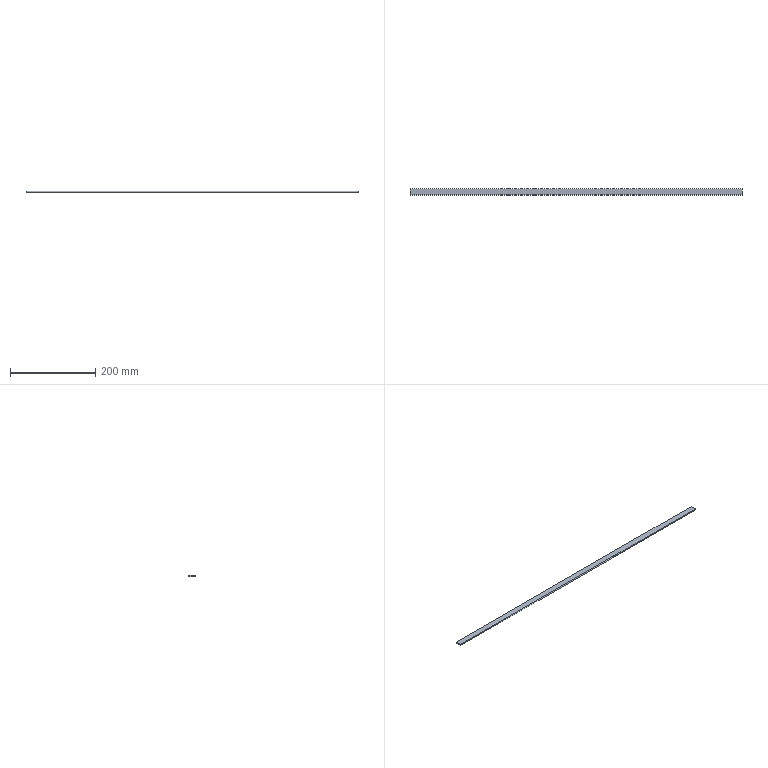Part | SolidWorks | features FlatPattern 1, Hem 1, SMBaseFlange 1, SheetMetal 1 | 1 solid | 14 faces | box 777 x 15 x 2.7 mm | volume 27651 mm3 | plane 12 | cylinder 2 | commonest cylinder face diameters 0.3 x1 2.7 x1
STEP:
#1=CARTESIAN_POINT('',(534.221,12.222,0.));
#2=VERTEX_POINT('',#1);
#3=CARTESIAN_POINT('',(534.221,25.872,0.));
#4=VERTEX_POINT('',#3);
#5=CARTESIAN_POINT('',(534.221,25.872,0.));
#6=DIRECTION('',(0.,1.,0.));
#7=VECTOR('',#6,1000.);
#8=LINE('',#5,#7);
#9=EDGE_CURVE('',#2,#4,#8,.T.);
#10=ORIENTED_EDGE('',*,*,#9,.F.);
#11=CARTESIAN_POINT('',(534.221,12.222,-1.2));
#12=VERTEX_POINT('',#11);
#13=CARTESIAN_POINT('',(534.221,12.222,0.));
#14=DIRECTION('',(0.,0.,-1.));
#15=VECTOR('',#14,1000.);
#16=LINE('',#13,#15);
#17=EDGE_CURVE('',#2,#12,#16,.T.);
#18=ORIENTED_EDGE('',*,*,#17,.T.);
#19=CARTESIAN_POINT('',(534.221,25.872,-1.2));
#20=VERTEX_POINT('',#19);
#21=CARTESIAN_POINT('',(534.221,25.872,-1.2));
#22=DIRECTION('',(0.,1.,0.));
#23=VECTOR('',#22,1000.);
#24=LINE('',#21,#23);
#25=EDGE_CURVE('',#12,#20,#24,.T.);
#26=ORIENTED_EDGE('',*,*,#25,.T.);
#27=CARTESIAN_POINT('',(534.221,25.872,-1.2));
#28=DIRECTION('',(0.,0.,1.));
#29=VECTOR('',#28,1000.);
#30=LINE('',#27,#29);
#31=EDGE_CURVE('',#20,#4,#30,.T.);
#32=ORIENTED_EDGE('',*,*,#31,.T.);
#33=EDGE_LOOP('',(#10,#18,#26,#32));
#34=FACE_OUTER_BOUND('',#33,.T.);
#35=CARTESIAN_POINT('',(534.221,25.872,-1.2));
#36=DIRECTION('',(1.,0.,0.));
#37=DIRECTION('',(0.,0.,-1.));
#38=AXIS2_PLACEMENT_3D('',#35,#36,#37);
#39=PLANE('',#38);
#40=ADVANCED_FACE('',(#34),#39,.T.);
#41=CARTESIAN_POINT('',(-242.779,12.222,0.));
#42=VERTEX_POINT('',#41);
#43=CARTESIAN_POINT('',(-242.779,12.222,-1.2));
#44=VERTEX_POINT('',#43);
#45=CARTESIAN_POINT('',(-242.779,12.222,0.));
#46=DIRECTION('',(0.,0.,-1.));
#47=VECTOR('',#46,1000.);
#48=LINE('',#45,#47);
#49=EDGE_CURVE('',#42,#44,#48,.T.);
#50=ORIENTED_EDGE('',*,*,#49,.F.);
#51=CARTESIAN_POINT('',(-242.779,25.872,0.));
#52=VERTEX_POINT('',#51);
#53=CARTESIAN_POINT('',(-242.779,25.872,0.));
#54=DIRECTION('',(0.,-1.,0.));
#55=VECTOR('',#54,1000.);
#56=LINE('',#53,#55);
#57=EDGE_CURVE('',#52,#42,#56,.T.);
#58=ORIENTED_EDGE('',*,*,#57,.F.);
#59=CARTESIAN_POINT('',(-242.779,25.872,-1.2));
#60=VERTEX_POINT('',#59);
#61=CARTESIAN_POINT('',(-242.779,25.872,-1.2));
#62=DIRECTION('',(0.,0.,1.));
#63=VECTOR('',#62,1000.);
#64=LINE('',#61,#63);
#65=EDGE_CURVE('',#60,#52,#64,.T.);
#66=ORIENTED_EDGE('',*,*,#65,.F.);
#67=CARTESIAN_POINT('',(-242.779,25.872,-1.2));
#68=DIRECTION('',(0.,-1.,0.));
#69=VECTOR('',#68,1000.);
#70=LINE('',#67,#69);
#71=EDGE_CURVE('',#60,#44,#70,.T.);
#72=ORIENTED_EDGE('',*,*,#71,.T.);
#73=EDGE_LOOP('',(#50,#58,#66,#72));
#74=FACE_OUTER_BOUND('',#73,.T.);
#75=CARTESIAN_POINT('',(-242.779,25.872,-1.2));
#76=DIRECTION('',(-1.,0.,0.));
#77=DIRECTION('',(0.,0.,1.));
#78=AXIS2_PLACEMENT_3D('',#75,#76,#77);
#79=PLANE('',#78);
#80=ADVANCED_FACE('',(#74),#79,.T.);
#81=CARTESIAN_POINT('',(-242.779,25.872,0.));
#82=DIRECTION('',(-1.,0.,0.));
#83=VECTOR('',#82,1000.);
#84=LINE('',#81,#83);
#85=EDGE_CURVE('',#4,#52,#84,.T.);
#86=ORIENTED_EDGE('',*,*,#85,.F.);
#87=ORIENTED_EDGE('',*,*,#31,.F.);
#88=CARTESIAN_POINT('',(-242.779,25.872,-1.2));
#89=DIRECTION('',(-1.,0.,0.));
#90=VECTOR('',#89,1000.);
#91=LINE('',#88,#90);
#92=EDGE_CURVE('',#20,#60,#91,.T.);
#93=ORIENTED_EDGE('',*,*,#92,.T.);
#94=ORIENTED_EDGE('',*,*,#65,.T.);
#95=EDGE_LOOP('',(#86,#87,#93,#94));
#96=FACE_OUTER_BOUND('',#95,.T.);
#97=CARTESIAN_POINT('',(-242.779,25.872,-1.2));
#98=DIRECTION('',(0.,1.,0.));
#99=DIRECTION('',(0.,0.,1.));
#100=AXIS2_PLACEMENT_3D('',#97,#98,#99);
#101=PLANE('',#100);
#102=ADVANCED_FACE('',(#96),#101,.T.);
#103=ORIENTED_EDGE('',*,*,#25,.F.);
#104=CARTESIAN_POINT('',(534.221,12.222,-1.2));
#105=DIRECTION('',(-1.,0.,0.));
#106=VECTOR('',#105,1000.);
#107=LINE('',#104,#106);
#108=EDGE_CURVE('',#12,#44,#107,.T.);
#109=ORIENTED_EDGE('',*,*,#108,.T.);
#110=ORIENTED_EDGE('',*,*,#71,.F.);
#111=ORIENTED_EDGE('',*,*,#92,.F.);
#112=EDGE_LOOP('',(#103,#109,#110,#111));
#113=FACE_OUTER_BOUND('',#112,.T.);
#114=CARTESIAN_POINT('',(0.,0.,-1.2));
#115=DIRECTION('',(0.,0.,1.));
#116=DIRECTION('',(1.,0.,0.));
#117=AXIS2_PLACEMENT_3D('',#114,#115,#116);
#118=PLANE('',#117);
#119=ADVANCED_FACE('',(#113),#118,.F.);
#120=CARTESIAN_POINT('',(534.221,12.222,0.));
#121=DIRECTION('',(-1.,0.,0.));
#122=VECTOR('',#121,1000.);
#123=LINE('',#120,#122);
#124=EDGE_CURVE('',#2,#42,#123,.T.);
#125=ORIENTED_EDGE('',*,*,#124,.F.);
#126=ORIENTED_EDGE('',*,*,#9,.T.);
#127=ORIENTED_EDGE('',*,*,#85,.T.);
#128=ORIENTED_EDGE('',*,*,#57,.T.);
#129=EDGE_LOOP('',(#125,#126,#127,#128));
#130=FACE_OUTER_BOUND('',#129,.T.);
#131=CARTESIAN_POINT('',(0.,0.,0.));
#132=DIRECTION('',(0.,0.,1.));
#133=DIRECTION('',(1.,0.,0.));
#134=AXIS2_PLACEMENT_3D('',#131,#132,#133);
#135=PLANE('',#134);
#136=ADVANCED_FACE('',(#130),#135,.T.);
#137=CARTESIAN_POINT('',(534.221,12.222,0.3));
#138=VERTEX_POINT('',#137);
#139=CARTESIAN_POINT('',(534.221,12.222,1.5));
#140=VERTEX_POINT('',#139);
#141=CARTESIAN_POINT('',(534.221,12.222,1.5));
#142=DIRECTION('',(0.,0.,1.));
#143=VECTOR('',#142,1000.);
#144=LINE('',#141,#143);
#145=EDGE_CURVE('',#138,#140,#144,.T.);
#146=ORIENTED_EDGE('',*,*,#145,.F.);
#147=CARTESIAN_POINT('',(534.221,25.872,0.3));
#148=VERTEX_POINT('',#147);
#149=CARTESIAN_POINT('',(534.221,19.047,0.3));
#150=DIRECTION('',(0.,-1.,0.));
#151=VECTOR('',#150,1000.);
#152=LINE('',#149,#151);
#153=EDGE_CURVE('',#148,#138,#152,.T.);
#154=ORIENTED_EDGE('',*,*,#153,.F.);
#155=CARTESIAN_POINT('',(534.221,25.872,1.5));
#156=VERTEX_POINT('',#155);
#157=CARTESIAN_POINT('',(534.221,25.872,1.5));
#158=DIRECTION('',(0.,0.,1.));
#159=VECTOR('',#158,1000.);
#160=LINE('',#157,#159);
#161=EDGE_CURVE('',#148,#156,#160,.T.);
#162=ORIENTED_EDGE('',*,*,#161,.T.);
#163=CARTESIAN_POINT('',(534.221,19.047,1.5));
#164=DIRECTION('',(0.,-1.,0.));
#165=VECTOR('',#164,1000.);
#166=LINE('',#163,#165);
#167=EDGE_CURVE('',#156,#140,#166,.T.);
#168=ORIENTED_EDGE('',*,*,#167,.T.);
#169=EDGE_LOOP('',(#146,#154,#162,#168));
#170=FACE_OUTER_BOUND('',#169,.T.);
#171=CARTESIAN_POINT('',(534.221,19.047,1.5));
#172=DIRECTION('',(-1.,0.,0.));
#173=DIRECTION('',(0.,-1.,0.));
#174=AXIS2_PLACEMENT_3D('',#171,#172,#173);
#175=PLANE('',#174);
#176=ADVANCED_FACE('',(#170),#175,.F.);
#177=ORIENTED_EDGE('',*,*,#161,.F.);
#178=CARTESIAN_POINT('',(-242.779,25.872,0.3));
#179=VERTEX_POINT('',#178);
#180=CARTESIAN_POINT('',(145.721,25.872,0.3));
#181=DIRECTION('',(1.,0.,0.));
#182=VECTOR('',#181,1000.);
#183=LINE('',#180,#182);
#184=EDGE_CURVE('',#179,#148,#183,.T.);
#185=ORIENTED_EDGE('',*,*,#184,.F.);
#186=CARTESIAN_POINT('',(-242.779,25.872,1.5));
#187=VERTEX_POINT('',#186);
#188=CARTESIAN_POINT('',(-242.779,25.872,1.5));
#189=DIRECTION('',(0.,0.,1.));
#190=VECTOR('',#189,1000.);
#191=LINE('',#188,#190);
#192=EDGE_CURVE('',#179,#187,#191,.T.);
#193=ORIENTED_EDGE('',*,*,#192,.T.);
#194=CARTESIAN_POINT('',(145.721,25.872,1.5));
#195=DIRECTION('',(1.,0.,0.));
#196=VECTOR('',#195,1000.);
#197=LINE('',#194,#196);
#198=EDGE_CURVE('',#187,#156,#197,.T.);
#199=ORIENTED_EDGE('',*,*,#198,.T.);
#200=EDGE_LOOP('',(#177,#185,#193,#199));
#201=FACE_OUTER_BOUND('',#200,.T.);
#202=CARTESIAN_POINT('',(145.721,25.872,1.5));
#203=DIRECTION('',(0.,-1.,0.));
#204=DIRECTION('',(1.,0.,0.));
#205=AXIS2_PLACEMENT_3D('',#202,#203,#204);
#206=PLANE('',#205);
#207=ADVANCED_FACE('',(#201),#206,.F.);
#208=CARTESIAN_POINT('',(-242.779,12.222,0.3));
#209=VERTEX_POINT('',#208);
#210=CARTESIAN_POINT('',(-242.779,19.047,0.3));
#211=DIRECTION('',(0.,1.,0.));
#212=VECTOR('',#211,1000.);
#213=LINE('',#210,#212);
#214=EDGE_CURVE('',#209,#179,#213,.T.);
#215=ORIENTED_EDGE('',*,*,#214,.F.);
#216=CARTESIAN_POINT('',(-242.779,12.222,1.5));
#217=VERTEX_POINT('',#216);
#218=CARTESIAN_POINT('',(-242.779,12.222,1.5));
#219=DIRECTION('',(0.,0.,1.));
#220=VECTOR('',#219,1000.);
#221=LINE('',#218,#220);
#222=EDGE_CURVE('',#209,#217,#221,.T.);
#223=ORIENTED_EDGE('',*,*,#222,.T.);
#224=CARTESIAN_POINT('',(-242.779,19.047,1.5));
#225=DIRECTION('',(0.,1.,0.));
#226=VECTOR('',#225,1000.);
#227=LINE('',#224,#226);
#228=EDGE_CURVE('',#217,#187,#227,.T.);
#229=ORIENTED_EDGE('',*,*,#228,.T.);
#230=ORIENTED_EDGE('',*,*,#192,.F.);
#231=EDGE_LOOP('',(#215,#223,#229,#230));
#232=FACE_OUTER_BOUND('',#231,.T.);
#233=CARTESIAN_POINT('',(-242.779,19.047,1.5));
#234=DIRECTION('',(1.,0.,0.));
#235=DIRECTION('',(0.,1.,0.));
#236=AXIS2_PLACEMENT_3D('',#233,#234,#235);
#237=PLANE('',#236);
#238=ADVANCED_FACE('',(#232),#237,.F.);
#239=ORIENTED_EDGE('',*,*,#198,.F.);
#240=ORIENTED_EDGE('',*,*,#228,.F.);
#241=CARTESIAN_POINT('',(145.721,12.222,1.5));
#242=DIRECTION('',(-1.,0.,0.));
#243=VECTOR('',#242,1000.);
#244=LINE('',#241,#243);
#245=EDGE_CURVE('',#140,#217,#244,.T.);
#246=ORIENTED_EDGE('',*,*,#245,.F.);
#247=ORIENTED_EDGE('',*,*,#167,.F.);
#248=EDGE_LOOP('',(#239,#240,#246,#247));
#249=FACE_OUTER_BOUND('',#248,.T.);
#250=CARTESIAN_POINT('',(145.721,19.047,1.5));
#251=DIRECTION('',(0.,0.,1.));
#252=DIRECTION('',(1.,0.,0.));
#253=AXIS2_PLACEMENT_3D('',#250,#251,#252);
#254=PLANE('',#253);
#255=ADVANCED_FACE('',(#249),#254,.T.);
#256=ORIENTED_EDGE('',*,*,#184,.T.);
#257=ORIENTED_EDGE('',*,*,#153,.T.);
#258=CARTESIAN_POINT('',(145.721,12.222,0.3));
#259=DIRECTION('',(-1.,0.,0.));
#260=VECTOR('',#259,1000.);
#261=LINE('',#258,#260);
#262=EDGE_CURVE('',#138,#209,#261,.T.);
#263=ORIENTED_EDGE('',*,*,#262,.T.);
#264=ORIENTED_EDGE('',*,*,#214,.T.);
#265=EDGE_LOOP('',(#256,#257,#263,#264));
#266=FACE_OUTER_BOUND('',#265,.T.);
#267=CARTESIAN_POINT('',(145.721,19.047,0.3));
#268=DIRECTION('',(0.,0.,1.));
#269=DIRECTION('',(1.,0.,0.));
#270=AXIS2_PLACEMENT_3D('',#267,#268,#269);
#271=PLANE('',#270);
#272=ADVANCED_FACE('',(#266),#271,.F.);
#273=ORIENTED_EDGE('',*,*,#222,.F.);
#274=CARTESIAN_POINT('',(-242.779,12.222,0.15));
#275=DIRECTION('',(-1.,0.,0.));
#276=DIRECTION('',(0.,0.,-1.));
#277=AXIS2_PLACEMENT_3D('',#274,#275,#276);
#278=CIRCLE('',#277,0.15);
#279=EDGE_CURVE('',#42,#209,#278,.T.);
#280=ORIENTED_EDGE('',*,*,#279,.F.);
#281=ORIENTED_EDGE('',*,*,#49,.T.);
#282=CARTESIAN_POINT('',(-242.779,12.222,0.15));
#283=DIRECTION('',(-1.,0.,0.));
#284=DIRECTION('',(0.,0.,-1.));
#285=AXIS2_PLACEMENT_3D('',#282,#283,#284);
#286=CIRCLE('',#285,1.35);
#287=EDGE_CURVE('',#44,#217,#286,.T.);
#288=ORIENTED_EDGE('',*,*,#287,.T.);
#289=EDGE_LOOP('',(#273,#280,#281,#288));
#290=FACE_OUTER_BOUND('',#289,.T.);
#291=CARTESIAN_POINT('',(-242.779,12.222,0.15));
#292=DIRECTION('',(-1.,0.,0.));
#293=DIRECTION('',(0.,0.,1.));
#294=AXIS2_PLACEMENT_3D('',#291,#292,#293);
#295=PLANE('',#294);
#296=ADVANCED_FACE('',(#290),#295,.T.);
#297=CARTESIAN_POINT('',(534.221,12.222,0.15));
#298=DIRECTION('',(1.,0.,0.));
#299=DIRECTION('',(0.,0.,-1.));
#300=AXIS2_PLACEMENT_3D('',#297,#298,#299);
#301=CIRCLE('',#300,0.15);
#302=EDGE_CURVE('',#138,#2,#301,.T.);
#303=ORIENTED_EDGE('',*,*,#302,.F.);
#304=ORIENTED_EDGE('',*,*,#145,.T.);
#305=CARTESIAN_POINT('',(534.221,12.222,0.15));
#306=DIRECTION('',(1.,0.,0.));
#307=DIRECTION('',(0.,0.,-1.));
#308=AXIS2_PLACEMENT_3D('',#305,#306,#307);
#309=CIRCLE('',#308,1.35);
#310=EDGE_CURVE('',#140,#12,#309,.T.);
#311=ORIENTED_EDGE('',*,*,#310,.T.);
#312=ORIENTED_EDGE('',*,*,#17,.F.);
#313=EDGE_LOOP('',(#303,#304,#311,#312));
#314=FACE_OUTER_BOUND('',#313,.T.);
#315=CARTESIAN_POINT('',(534.221,12.222,0.15));
#316=DIRECTION('',(-1.,0.,0.));
#317=DIRECTION('',(0.,0.,1.));
#318=AXIS2_PLACEMENT_3D('',#315,#316,#317);
#319=PLANE('',#318);
#320=ADVANCED_FACE('',(#314),#319,.F.);
#321=ORIENTED_EDGE('',*,*,#108,.F.);
#322=ORIENTED_EDGE('',*,*,#310,.F.);
#323=ORIENTED_EDGE('',*,*,#245,.T.);
#324=ORIENTED_EDGE('',*,*,#287,.F.);
#325=EDGE_LOOP('',(#321,#322,#323,#324));
#326=FACE_OUTER_BOUND('',#325,.T.);
#327=CARTESIAN_POINT('',(534.221,12.222,0.15));
#328=DIRECTION('',(1.,0.,0.));
#329=DIRECTION('',(0.,0.,1.));
#330=AXIS2_PLACEMENT_3D('',#327,#328,#329);
#331=CYLINDRICAL_SURFACE('',#330,1.35);
#332=ADVANCED_FACE('',(#326),#331,.T.);
#333=ORIENTED_EDGE('',*,*,#124,.T.);
#334=ORIENTED_EDGE('',*,*,#279,.T.);
#335=ORIENTED_EDGE('',*,*,#262,.F.);
#336=ORIENTED_EDGE('',*,*,#302,.T.);
#337=EDGE_LOOP('',(#333,#334,#335,#336));
#338=FACE_OUTER_BOUND('',#337,.T.);
#339=CARTESIAN_POINT('',(534.221,12.222,0.15));
#340=DIRECTION('',(1.,0.,0.));
#341=DIRECTION('',(0.,0.,1.));
#342=AXIS2_PLACEMENT_3D('',#339,#340,#341);
#343=CYLINDRICAL_SURFACE('',#342,0.15);
#344=ADVANCED_FACE('',(#338),#343,.F.);
#345=CLOSED_SHELL('',(#40,#80,#102,#119,#136,#176,#207,#238,#255,#272,#296,#320,#332,#344));
#346=MANIFOLD_SOLID_BREP('',#345);
#347=CARTESIAN_POINT('',(0.,0.,0.));
#348=DIRECTION('',(0.,0.,1.));
#349=DIRECTION('',(1.,0.,0.));
#350=AXIS2_PLACEMENT_3D('',#347,#348,#349);
#351=(LENGTH_UNIT()NAMED_UNIT(*)SI_UNIT(.MILLI.,.METRE.));
#352=UNCERTAINTY_MEASURE_WITH_UNIT(LENGTH_MEASURE(0.00001),#351,'','');
#353=(NAMED_UNIT(*)PLANE_ANGLE_UNIT()SI_UNIT($,.RADIAN.));
#354=(NAMED_UNIT(*)SI_UNIT($,.STERADIAN.)SOLID_ANGLE_UNIT());
#355=(GEOMETRIC_REPRESENTATION_CONTEXT(3)GLOBAL_UNCERTAINTY_ASSIGNED_CONTEXT((#352))GLOBAL_UNIT_ASSIGNED_CONTEXT((#351,#353,#354))REPRESENTATION_CONTEXT('',''));
#356=ADVANCED_BREP_SHAPE_REPRESENTATION('',(#346,#350),#355);